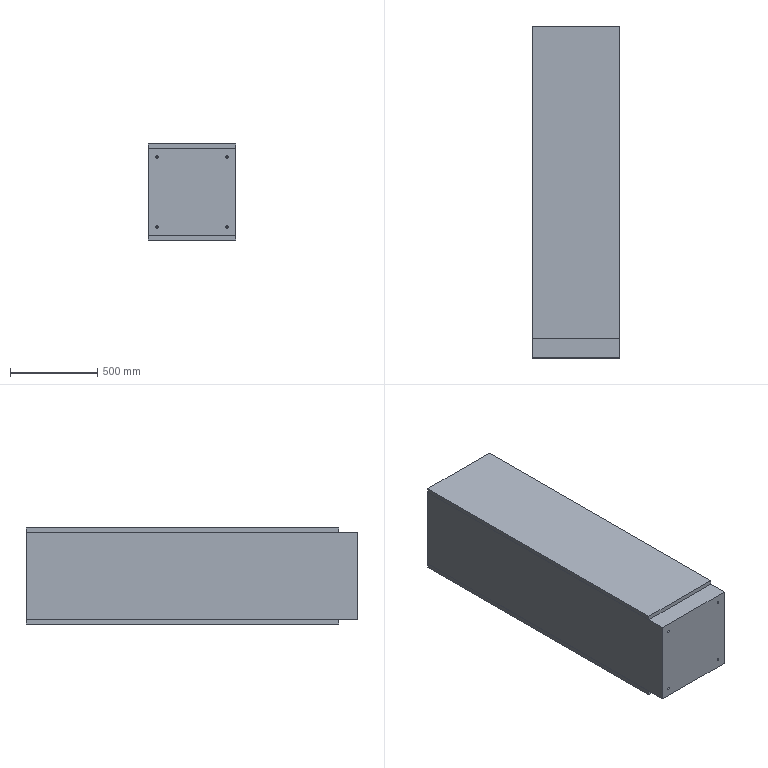Part | STEP file | Air conditioner cabinet | 3 solids | 256 faces | box 500 x 1900 x 550 mm | volume 519606146 mm3 | plane 129 | spline 119 | cylinder 8 | commonest cylinder face diameters 14 x8